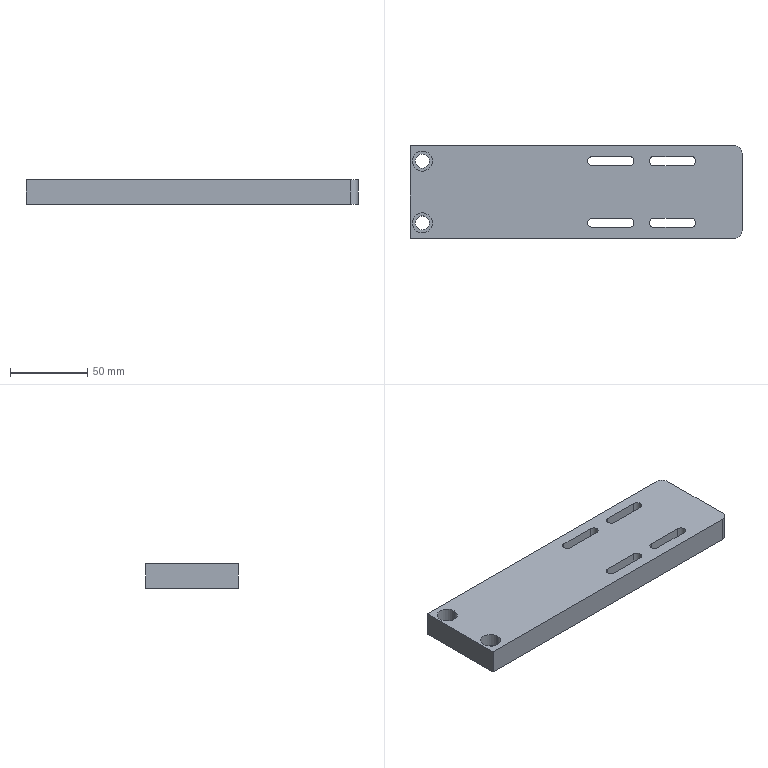NC program | Mastercam | posted with a generic post | part box 215 x 60 x 16 mm
Lines 5150 to 6620 of 6620, first 1383 of 1471 lines:
N1990 T7 M6
N2000 G0 G90 G17 G54 X-99.5 Y-20. A0. S3000 M3
N2010 G43 H7 Z50. M8
N2020 G98 G81 Z-.7 R1. F300.
N2030 Y20.
N2040 X10.5
N2050 X34.5
N2060 X50.5
N2070 X74.5
N2080 Y-20.
N2090 X50.5
N2100 X34.5
N2110 X10.5
N2120 G80
N2130 M5
N2140 G91 G0 G28 Z0. M9
N2150 A0.
N2160 M01
N2170 T1 M6
N2180 G0 G90 G17 G54 X-99.5 Y-20. A0. S2000 M3
N2190 G43 H1 Z50. M8
N2200 G98 G83 Z-18.902 R1. Q3. F200.
N2210 Y20.
N2220 X10.5
N2230 X34.5
N2240 X50.5
N2250 X74.5
N2260 Y-20.
N2270 X50.5
N2280 X34.5
N2290 X10.5
N2300 G80
N2310 M5
N2320 G91 G0 G28 Z0. M9
N2330 A0.
N2340 M01
N2350 T6 M6
N2360 G0 G90 G17 G54 X-99.5 Y20. A0. S7000 M3
N2370 G43 H6 Z50. M8
N2380 Z5.
N2390 G1 Z0. F600.
N2400 X-97.8 Y21.7 F3000.
N2410 G3 X-99.5 Y23.4 I-1.7 J0.
N2420 X-102.9 Y20. Z-.125 I0. J-3.4
N2430 X-99.5 Y16.6 Z-.25 I3.4 J0.
N2440 X-96.1 Y20. Z-.375 I0. J3.4
N2450 X-99.5 Y23.4 Z-.5 I-3.4 J0.
N2460 X-102.9 Y20. Z-.625 I0. J-3.4
N2470 X-99.5 Y16.6 Z-.75 I3.4 J0.
N2480 X-96.1 Y20. Z-.875 I0. J3.4
N2490 X-99.5 Y23.4 Z-1. I-3.4 J0.
N2500 X-102.9 Y20. Z-1.125 I0. J-3.4
N2510 X-99.5 Y16.6 Z-1.25 I3.4 J0.
N2520 X-96.1 Y20. Z-1.375 I0. J3.4
N2530 X-99.5 Y23.4 Z-1.5 I-3.4 J0.
N2540 X-102.9 Y20. Z-1.625 I0. J-3.4
N2550 X-99.5 Y16.6 Z-1.75 I3.4 J0.
N2560 X-96.1 Y20. Z-1.875 I0. J3.4
N2570 X-99.5 Y23.4 Z-2. I-3.4 J0.
N2580 X-102.9 Y20. Z-2.125 I0. J-3.4
N2590 X-99.5 Y16.6 Z-2.25 I3.4 J0.
N2600 X-96.1 Y20. Z-2.375 I0. J3.4
N2610 X-99.5 Y23.4 Z-2.5 I-3.4 J0.
N2620 X-102.9 Y20. Z-2.625 I0. J-3.4
N2630 X-99.5 Y16.6 Z-2.75 I3.4 J0.
N2640 X-96.1 Y20. Z-2.875 I0. J3.4
N2650 X-99.5 Y23.4 Z-3. I-3.4 J0.
N2660 X-102.9 Y20. Z-3.125 I0. J-3.4
N2670 X-99.5 Y16.6 Z-3.25 I3.4 J0.
N2680 X-96.1 Y20. Z-3.375 I0. J3.4
N2690 X-99.5 Y23.4 Z-3.5 I-3.4 J0.
N2700 X-102.9 Y20. Z-3.625 I0. J-3.4
N2710 X-99.5 Y16.6 Z-3.75 I3.4 J0.
N2720 X-96.1 Y20. Z-3.875 I0. J3.4
N2730 X-99.5 Y23.4 Z-4. I-3.4 J0.
N2740 X-102.9 Y20. Z-4.125 I0. J-3.4
N2750 X-99.5 Y16.6 Z-4.25 I3.4 J0.
N2760 X-96.1 Y20. Z-4.375 I0. J3.4
N2770 X-99.5 Y23.4 Z-4.5 I-3.4 J0.
N2780 X-102.9 Y20. Z-4.625 I0. J-3.4
N2790 X-99.5 Y16.6 Z-4.75 I3.4 J0.
N2800 X-96.1 Y20. Z-4.875 I0. J3.4
N2810 X-99.5 Y23.4 Z-5. I-3.4 J0.
N2820 X-102.9 Y20. Z-5.125 I0. J-3.4
N2830 X-99.5 Y16.6 Z-5.25 I3.4 J0.
N2840 X-96.1 Y20. Z-5.375 I0. J3.4
N2850 X-99.5 Y23.4 Z-5.5 I-3.4 J0.
N2860 X-102.9 Y20. Z-5.625 I0. J-3.4
N2870 X-99.5 Y16.6 Z-5.75 I3.4 J0.
N2880 X-96.1 Y20. Z-5.875 I0. J3.4
N2890 X-99.5 Y23.4 Z-6. I-3.4 J0.
N2900 X-102.9 Y20. Z-6.125 I0. J-3.4
N2910 X-99.5 Y16.6 Z-6.25 I3.4 J0.
N2920 X-96.1 Y20. Z-6.375 I0. J3.4
N2930 X-99.5 Y23.4 Z-6.5 I-3.4 J0.
N2940 X-102.9 Y20. Z-6.625 I0. J-3.4
N2950 X-99.5 Y16.6 Z-6.75 I3.4 J0.
N2960 X-96.1 Y20. Z-6.875 I0. J3.4
N2970 X-99.5 Y23.4 Z-7. I-3.4 J0.
N2980 X-102.9 Y20. Z-7.125 I0. J-3.4
N2990 X-99.5 Y16.6 Z-7.25 I3.4 J0.
N3000 X-96.1 Y20. Z-7.375 I0. J3.4
N3010 X-99.5 Y23.4 Z-7.5 I-3.4 J0.
N3020 X-102.9 Y20. Z-7.625 I0. J-3.4
N3030 X-99.5 Y16.6 Z-7.75 I3.4 J0.
N3040 X-96.1 Y20. Z-7.875 I0. J3.4
N3050 X-99.5 Y23.4 Z-8. I-3.4 J0.
N3060 X-102.9 Y20. Z-8.125 I0. J-3.4
N3070 X-99.5 Y16.6 Z-8.25 I3.4 J0.
N3080 X-96.1 Y20. Z-8.375 I0. J3.4
N3090 X-99.5 Y23.4 Z-8.5 I-3.4 J0.
N3100 X-102.9 Y20. Z-8.625 I0. J-3.4
N3110 X-99.5 Y16.6 Z-8.75 I3.4 J0.
N3120 X-96.1 Y20. Z-8.875 I0. J3.4
N3130 X-99.5 Y23.4 Z-9. I-3.4 J0.
N3140 X-102.9 Y20. I0. J-3.4 F900.
N3150 X-99.5 Y16.6 I3.4 J0.
N3160 X-96.1 Y20. I0. J3.4
N3170 X-99.5 Y23.4 I-3.4 J0.
N3180 X-100.486 Y23.254 I0. J-3.4
N3190 X-101.693 Y21.627 I.493 J-1.627
N3200 X-101.62 Y21.134 I1.7 J0.
N3210 G1 X-99.5 Y20.
N3220 G0 Z0.
N3230 G1 X-97.75 Y21.75 F1000.
N3240 G3 X-99.5 Y23.5 I-1.75 J0.
N3250 X-103. Y20. I0. J-3.5
N3260 X-99.5 Y16.5 I3.5 J0.
N3270 X-96. Y20. I0. J3.5
N3280 X-99.5 Y23.5 I-3.5 J0.
N3290 X-100.486 Y23.358 I0. J-3.5
N3300 X-103. Y20. Z-1.023 I.986 J-3.358
N3310 X-99.5 Y16.5 Z-2.273 I3.5 J0.
N3320 X-96. Y20. Z-3.523 I0. J3.5
N3330 X-99.5 Y23.5 Z-4.773 I-3.5 J0.
N3340 X-100.486 Y23.358 Z-5. I0. J-3.5
N3350 X-103. Y20. Z-6.023 I.986 J-3.358
N3360 X-99.5 Y16.5 Z-7.273 I3.5 J0.
N3370 X-96. Y20. Z-8.523 I0. J3.5
N3380 X-96.611 Y21.976 Z-9. I-3.5 J0.
N3390 X-99.5 Y23.5 I-2.889 J-1.976
N3400 X-103. Y20. I0. J-3.5
N3410 X-99.5 Y16.5 I3.5 J0.
N3420 X-96. Y20. I0. J3.5
N3430 X-96.611 Y21.976 I-3.5 J0.
N3440 X-97.285 Y22.71 I-2.889 J-1.976
N3450 X-98.393 Y23.105 I-1.108 J-1.355
N3460 X-99.748 Y22.462 I0. J-1.75
N3470 G1 X-99.5 Y20.
N3480 G0 Z50.
N3490 Y-20.
N3500 Z5.
N3510 G1 Z0. F600.
N3520 X-97.8 Y-18.3 F3000.
N3530 G3 X-99.5 Y-16.6 I-1.7 J0.
N3540 X-102.9 Y-20. Z-.125 I0. J-3.4
N3550 X-99.5 Y-23.4 Z-.25 I3.4 J0.
N3560 X-96.1 Y-20. Z-.375 I0. J3.4
N3570 X-99.5 Y-16.6 Z-.5 I-3.4 J0.
N3580 X-102.9 Y-20. Z-.625 I0. J-3.4
N3590 X-99.5 Y-23.4 Z-.75 I3.4 J0.
N3600 X-96.1 Y-20. Z-.875 I0. J3.4
N3610 X-99.5 Y-16.6 Z-1. I-3.4 J0.
N3620 X-102.9 Y-20. Z-1.125 I0. J-3.4
N3630 X-99.5 Y-23.4 Z-1.25 I3.4 J0.
N3640 X-96.1 Y-20. Z-1.375 I0. J3.4
N3650 X-99.5 Y-16.6 Z-1.5 I-3.4 J0.
N3660 X-102.9 Y-20. Z-1.625 I0. J-3.4
N3670 X-99.5 Y-23.4 Z-1.75 I3.4 J0.
N3680 X-96.1 Y-20. Z-1.875 I0. J3.4
N3690 X-99.5 Y-16.6 Z-2. I-3.4 J0.
N3700 X-102.9 Y-20. Z-2.125 I0. J-3.4
N3710 X-99.5 Y-23.4 Z-2.25 I3.4 J0.
N3720 X-96.1 Y-20. Z-2.375 I0. J3.4
N3730 X-99.5 Y-16.6 Z-2.5 I-3.4 J0.
N3740 X-102.9 Y-20. Z-2.625 I0. J-3.4
N3750 X-99.5 Y-23.4 Z-2.75 I3.4 J0.
N3760 X-96.1 Y-20. Z-2.875 I0. J3.4
N3770 X-99.5 Y-16.6 Z-3. I-3.4 J0.
N3780 X-102.9 Y-20. Z-3.125 I0. J-3.4
N3790 X-99.5 Y-23.4 Z-3.25 I3.4 J0.
N3800 X-96.1 Y-20. Z-3.375 I0. J3.4
N3810 X-99.5 Y-16.6 Z-3.5 I-3.4 J0.
N3820 X-102.9 Y-20. Z-3.625 I0. J-3.4
N3830 X-99.5 Y-23.4 Z-3.75 I3.4 J0.
N3840 X-96.1 Y-20. Z-3.875 I0. J3.4
N3850 X-99.5 Y-16.6 Z-4. I-3.4 J0.
N3860 X-102.9 Y-20. Z-4.125 I0. J-3.4
N3870 X-99.5 Y-23.4 Z-4.25 I3.4 J0.
N3880 X-96.1 Y-20. Z-4.375 I0. J3.4
N3890 X-99.5 Y-16.6 Z-4.5 I-3.4 J0.
N3900 X-102.9 Y-20. Z-4.625 I0. J-3.4
N3910 X-99.5 Y-23.4 Z-4.75 I3.4 J0.
N3920 X-96.1 Y-20. Z-4.875 I0. J3.4
N3930 X-99.5 Y-16.6 Z-5. I-3.4 J0.
N3940 X-102.9 Y-20. Z-5.125 I0. J-3.4
N3950 X-99.5 Y-23.4 Z-5.25 I3.4 J0.
N3960 X-96.1 Y-20. Z-5.375 I0. J3.4
N3970 X-99.5 Y-16.6 Z-5.5 I-3.4 J0.
N3980 X-102.9 Y-20. Z-5.625 I0. J-3.4
N3990 X-99.5 Y-23.4 Z-5.75 I3.4 J0.
N4000 X-96.1 Y-20. Z-5.875 I0. J3.4
N4010 X-99.5 Y-16.6 Z-6. I-3.4 J0.
N4020 X-102.9 Y-20. Z-6.125 I0. J-3.4
N4030 X-99.5 Y-23.4 Z-6.25 I3.4 J0.
N4040 X-96.1 Y-20. Z-6.375 I0. J3.4
N4050 X-99.5 Y-16.6 Z-6.5 I-3.4 J0.
N4060 X-102.9 Y-20. Z-6.625 I0. J-3.4
N4070 X-99.5 Y-23.4 Z-6.75 I3.4 J0.
N4080 X-96.1 Y-20. Z-6.875 I0. J3.4
N4090 X-99.5 Y-16.6 Z-7. I-3.4 J0.
N4100 X-102.9 Y-20. Z-7.125 I0. J-3.4
N4110 X-99.5 Y-23.4 Z-7.25 I3.4 J0.
N4120 X-96.1 Y-20. Z-7.375 I0. J3.4
N4130 X-99.5 Y-16.6 Z-7.5 I-3.4 J0.
N4140 X-102.9 Y-20. Z-7.625 I0. J-3.4
N4150 X-99.5 Y-23.4 Z-7.75 I3.4 J0.
N4160 X-96.1 Y-20. Z-7.875 I0. J3.4
N4170 X-99.5 Y-16.6 Z-8. I-3.4 J0.
N4180 X-102.9 Y-20. Z-8.125 I0. J-3.4
N4190 X-99.5 Y-23.4 Z-8.25 I3.4 J0.
N4200 X-96.1 Y-20. Z-8.375 I0. J3.4
N4210 X-99.5 Y-16.6 Z-8.5 I-3.4 J0.
N4220 X-102.9 Y-20. Z-8.625 I0. J-3.4
N4230 X-99.5 Y-23.4 Z-8.75 I3.4 J0.
N4240 X-96.1 Y-20. Z-8.875 I0. J3.4
N4250 X-99.5 Y-16.6 Z-9. I-3.4 J0.
N4260 X-102.9 Y-20. I0. J-3.4 F900.
N4270 X-99.5 Y-23.4 I3.4 J0.
N4280 X-96.1 Y-20. I0. J3.4
N4290 X-99.5 Y-16.6 I-3.4 J0.
N4300 X-100.486 Y-16.746 I0. J-3.4
N4310 X-101.693 Y-18.373 I.493 J-1.627
N4320 X-101.62 Y-18.866 I1.7 J0.
N4330 G1 X-99.5 Y-20.
N4340 G0 Z0.
N4350 G1 X-97.75 Y-18.25 F1000.
N4360 G3 X-99.5 Y-16.5 I-1.75 J0.
N4370 X-103. Y-20. I0. J-3.5
N4380 X-99.5 Y-23.5 I3.5 J0.
N4390 X-96. Y-20. I0. J3.5
N4400 X-99.5 Y-16.5 I-3.5 J0.
N4410 X-100.486 Y-16.642 I0. J-3.5
N4420 X-103. Y-20. Z-1.023 I.986 J-3.358
N4430 X-99.5 Y-23.5 Z-2.273 I3.5 J0.
N4440 X-96. Y-20. Z-3.523 I0. J3.5
N4450 X-99.5 Y-16.5 Z-4.773 I-3.5 J0.
N4460 X-100.486 Y-16.642 Z-5. I0. J-3.5
N4470 X-103. Y-20. Z-6.023 I.986 J-3.358
N4480 X-99.5 Y-23.5 Z-7.273 I3.5 J0.
N4490 X-96. Y-20. Z-8.523 I0. J3.5
N4500 X-96.611 Y-18.024 Z-9. I-3.5 J0.
N4510 X-99.5 Y-16.5 I-2.889 J-1.976
N4520 X-103. Y-20. I0. J-3.5
N4530 X-99.5 Y-23.5 I3.5 J0.
N4540 X-96. Y-20. I0. J3.5
N4550 X-96.611 Y-18.024 I-3.5 J0.
N4560 X-97.285 Y-17.29 I-2.889 J-1.976
N4570 X-98.393 Y-16.895 I-1.108 J-1.355
N4580 X-99.748 Y-17.538 I0. J-1.75
N4590 G1 X-99.5 Y-20.
N4600 G0 Z50.
N4610 M5
N4620 G91 G28 Z0. M9
N4630 A0.
N4640 M01
N4650 T5 M6
N4660 G0 G90 G17 G54 X10.5 Y20. A0. S7000 M3
N4670 G43 H5 Z25. M8
N4680 Z1.
N4690 G1 Z-.5 F600.
N4700 X34.5 F3000.
N4710 Z-1. F600.
N4720 X10.5 F3000.
N4730 Z-1.5 F600.
N4740 X34.5 F3000.
N4750 Z-2. F600.
N4760 X10.5 F3000.
N4770 Z-2.5 F600.
N4780 X34.5 F3000.
N4790 Z-3. F600.
N4800 X10.5 F3000.
N4810 Z-3.5 F600.
N4820 X34.5 F3000.
N4830 Z-4. F600.
N4840 X10.5 F3000.
N4850 Z-4.5 F600.
N4860 X34.5 F3000.
N4870 Z-5. F600.
N4880 X10.5 F3000.
N4890 Z-5.5 F600.
N4900 X34.5 F3000.
N4910 Z-6. F600.
N4920 X10.5 F3000.
N4930 Z-6.5 F600.
N4940 X34.5 F3000.
N4950 Z-7. F600.
N4960 X10.5 F3000.
N4970 Z-7.5 F600.
N4980 X34.5 F3000.
N4990 Z-8. F600.
N5000 X10.5 F3000.
N5010 Z-8.5 F600.
N5020 X34.5 F3000.
N5030 Z-9. F600.
N5040 X10.5 F3000.
N5050 Z-9.5 F600.
N5060 X34.5 F3000.
N5070 Z-10. F600.
N5080 X10.5 F3000.
N5090 Z-10.5 F600.
N5100 X34.5 F3000.
N5110 Z-11. F600.
N5120 X10.5 F3000.
N5130 Z-11.5 F600.
N5140 X34.5 F3000.
N5150 Z-12. F600.
N5160 X10.5 F3000.
N5170 Z-12.5 F600.
N5180 X34.5 F3000.
N5190 Z-13. F600.
N5200 X10.5 F3000.
N5210 Z-13.5 F600.
N5220 X34.5 F3000.
N5230 Z-14. F600.
N5240 X10.5 F3000.
N5250 Z-14.5 F600.
N5260 X34.5 F3000.
N5270 Z-15. F600.
N5280 X10.5 F3000.
N5290 Z-15.5 F600.
N5300 X34.5 F3000.
N5310 Z-16. F600.
N5320 X10.5 F3000.
N5330 Z-16.5 F600.
N5340 X34.5 F3000.
N5350 Z-17. F600.
N5360 X10.5 F3000.
N5370 G0 Z25.
N5380 X50.5
N5390 Z1.
N5400 G1 Z-.5 F600.
N5410 X74.5 F3000.
N5420 Z-1. F600.
N5430 X50.5 F3000.
N5440 Z-1.5 F600.
N5450 X74.5 F3000.
N5460 Z-2. F600.
N5470 X50.5 F3000.
N5480 Z-2.5 F600.
N5490 X74.5 F3000.
N5500 Z-3. F600.
N5510 X50.5 F3000.
N5520 Z-3.5 F600.
N5530 X74.5 F3000.
N5540 Z-4. F600.
N5550 X50.5 F3000.
N5560 Z-4.5 F600.
N5570 X74.5 F3000.
N5580 Z-5. F600.
N5590 X50.5 F3000.
N5600 Z-5.5 F600.
N5610 X74.5 F3000.
N5620 Z-6. F600.
N5630 X50.5 F3000.
N5640 Z-6.5 F600.
N5650 X74.5 F3000.
N5660 Z-7. F600.
N5670 X50.5 F3000.
N5680 Z-7.5 F600.
N5690 X74.5 F3000.
N5700 Z-8. F600.
N5710 X50.5 F3000.
N5720 Z-8.5 F600.
N5730 X74.5 F3000.
N5740 Z-9. F600.
N5750 X50.5 F3000.
N5760 Z-9.5 F600.
N5770 X74.5 F3000.
N5780 Z-10. F600.
N5790 X50.5 F3000.
N5800 Z-10.5 F600.
N5810 X74.5 F3000.
N5820 Z-11. F600.
N5830 X50.5 F3000.
N5840 Z-11.5 F600.
N5850 X74.5 F3000.
N5860 Z-12. F600.
N5870 X50.5 F3000.
N5880 Z-12.5 F600.
N5890 X74.5 F3000.
N5900 Z-13. F600.
N5910 X50.5 F3000.
N5920 Z-13.5 F600.
N5930 X74.5 F3000.
N5940 Z-14. F600.
N5950 X50.5 F3000.
N5960 Z-14.5 F600.
N5970 X74.5 F3000.
N5980 Z-15. F600.
N5990 X50.5 F3000.
N6000 Z-15.5 F600.
N6010 X74.5 F3000.
N6020 Z-16. F600.
N6030 X50.5 F3000.
N6040 Z-16.5 F600.
N6050 X74.5 F3000.
N6060 Z-17. F600.
N6070 X50.5 F3000.
N6080 G0 Z25.
N6090 X10.5 Y-20.
N6100 Z1.
N6110 G1 Z-.5 F600.
N6120 X34.5 F3000.
N6130 Z-1. F600.
N6140 X10.5 F3000.
N6150 Z-1.5 F600.
N6160 X34.5 F3000.
N6170 Z-2. F600.
N6180 X10.5 F3000.
N6190 Z-2.5 F600.
N6200 X34.5 F3000.
N6210 Z-3. F600.
N6220 X10.5 F3000.
N6230 Z-3.5 F600.
N6240 X34.5 F3000.
N6250 Z-4. F600.
N6260 X10.5 F3000.
N6270 Z-4.5 F600.
N6280 X34.5 F3000.
N6290 Z-5. F600.
N6300 X10.5 F3000.
N6310 Z-5.5 F600.
N6320 X34.5 F3000.
N6330 Z-6. F600.
N6340 X10.5 F3000.
N6350 Z-6.5 F600.
N6360 X34.5 F3000.
N6370 Z-7. F600.
N6380 X10.5 F3000.
N6390 Z-7.5 F600.
N6400 X34.5 F3000.
N6410 Z-8. F600.
N6420 X10.5 F3000.
N6430 Z-8.5 F600.
N6440 X34.5 F3000.
N6450 Z-9. F600.
N6460 X10.5 F3000.
N6470 Z-9.5 F600.
N6480 X34.5 F3000.
N6490 Z-10. F600.
N6500 X10.5 F3000.
N6510 Z-10.5 F600.
N6520 X34.5 F3000.
N6530 Z-11. F600.
N6540 X10.5 F3000.
N6550 Z-11.5 F600.
N6560 X34.5 F3000.
N6570 Z-12. F600.
N6580 X10.5 F3000.
N6590 Z-12.5 F600.
N6600 X34.5 F3000.
N6610 Z-13. F600.
N6620 X10.5 F3000.
N6630 Z-13.5 F600.
N6640 X34.5 F3000.
N6650 Z-14. F600.
N6660 X10.5 F3000.
N6670 Z-14.5 F600.
N6680 X34.5 F3000.
N6690 Z-15. F600.
N6700 X10.5 F3000.
N6710 Z-15.5 F600.
N6720 X34.5 F3000.
N6730 Z-16. F600.
N6740 X10.5 F3000.
N6750 Z-16.5 F600.
N6760 X34.5 F3000.
N6770 Z-17. F600.
N6780 X10.5 F3000.
N6790 G0 Z25.
N6800 X50.5
N6810 Z1.
N6820 G1 Z-.5 F600.
N6830 X74.5 F3000.
N6840 Z-1. F600.
N6850 X50.5 F3000.
N6860 Z-1.5 F600.
N6870 X74.5 F3000.
N6880 Z-2. F600.
N6890 X50.5 F3000.
N6900 Z-2.5 F600.
N6910 X74.5 F3000.
N6920 Z-3. F600.
N6930 X50.5 F3000.
N6940 Z-3.5 F600.
N6950 X74.5 F3000.
N6960 Z-4. F600.
N6970 X50.5 F3000.
N6980 Z-4.5 F600.
N6990 X74.5 F3000.
N7000 Z-5. F600.
N7010 X50.5 F3000.
N7020 Z-5.5 F600.
N7030 X74.5 F3000.
N7040 Z-6. F600.
N7050 X50.5 F3000.
N7060 Z-6.5 F600.
N7070 X74.5 F3000.
N7080 Z-7. F600.
N7090 X50.5 F3000.
N7100 Z-7.5 F600.
N7110 X74.5 F3000.
N7120 Z-8. F600.
N7130 X50.5 F3000.
N7140 Z-8.5 F600.
N7150 X74.5 F3000.
N7160 Z-9. F600.
N7170 X50.5 F3000.
N7180 Z-9.5 F600.
N7190 X74.5 F3000.
N7200 Z-10. F600.
N7210 X50.5 F3000.
N7220 Z-10.5 F600.
N7230 X74.5 F3000.
N7240 Z-11. F600.
N7250 X50.5 F3000.
N7260 Z-11.5 F600.
N7270 X74.5 F3000.
N7280 Z-12. F600.
N7290 X50.5 F3000.
N7300 Z-12.5 F600.
N7310 X74.5 F3000.
N7320 Z-13. F600.
N7330 X50.5 F3000.
N7340 Z-13.5 F600.
N7350 X74.5 F3000.
N7360 Z-14. F600.
N7370 X50.5 F3000.
N7380 Z-14.5 F600.
N7390 X74.5 F3000.
N7400 Z-15. F600.
N7410 X50.5 F3000.
N7420 Z-15.5 F600.
N7430 X74.5 F3000.
N7440 Z-16. F600.
N7450 X50.5 F3000.
N7460 Z-16.5 F600.
N7470 X74.5 F3000.
N7480 Z-17. F600.
N7490 X50.5 F3000.
N7500 G0 Z25.
N7510 X-99.5 Y20. Z41.
N7520 Z-4.
N7530 G1 Z-9. F600.
N7540 X-98.55 Y20.95 F3000.
N7550 G3 X-99.5 Y21.9 I-.95 J0.
N7560 X-101.4 Y20. Z-9.125 I0. J-1.9
N7570 X-99.5 Y18.1 Z-9.25 I1.9 J0.
N7580 X-97.6 Y20. Z-9.375 I0. J1.9
N7590 X-99.5 Y21.9 Z-9.5 I-1.9 J0.
N7600 X-101.4 Y20. Z-9.625 I0. J-1.9
N7610 X-99.5 Y18.1 Z-9.75 I1.9 J0.
N7620 X-97.6 Y20. Z-9.875 I0. J1.9
N7630 X-99.5 Y21.9 Z-10. I-1.9 J0.
N7640 X-101.4 Y20. Z-10.125 I0. J-1.9
N7650 X-99.5 Y18.1 Z-10.25 I1.9 J0.
N7660 X-97.6 Y20. Z-10.375 I0. J1.9
N7670 X-99.5 Y21.9 Z-10.5 I-1.9 J0.
N7680 X-101.4 Y20. Z-10.625 I0. J-1.9
N7690 X-99.5 Y18.1 Z-10.75 I1.9 J0.
N7700 X-97.6 Y20. Z-10.875 I0. J1.9
N7710 X-99.5 Y21.9 Z-11. I-1.9 J0.
N7720 X-101.4 Y20. Z-11.125 I0. J-1.9
N7730 X-99.5 Y18.1 Z-11.25 I1.9 J0.
N7740 X-97.6 Y20. Z-11.375 I0. J1.9
N7750 X-99.5 Y21.9 Z-11.5 I-1.9 J0.
N7760 X-101.4 Y20. Z-11.625 I0. J-1.9
N7770 X-99.5 Y18.1 Z-11.75 I1.9 J0.
N7780 X-97.6 Y20. Z-11.875 I0. J1.9
N7790 X-99.5 Y21.9 Z-12. I-1.9 J0.
N7800 X-101.4 Y20. Z-12.125 I0. J-1.9
N7810 X-99.5 Y18.1 Z-12.25 I1.9 J0.
N7820 X-97.6 Y20. Z-12.375 I0. J1.9
N7830 X-99.5 Y21.9 Z-12.5 I-1.9 J0.
N7840 X-101.4 Y20. Z-12.625 I0. J-1.9
N7850 X-99.5 Y18.1 Z-12.75 I1.9 J0.
N7860 X-97.6 Y20. Z-12.875 I0. J1.9
N7870 X-99.5 Y21.9 Z-13. I-1.9 J0.
N7880 X-101.4 Y20. Z-13.125 I0. J-1.9
N7890 X-99.5 Y18.1 Z-13.25 I1.9 J0.
N7900 X-97.6 Y20. Z-13.375 I0. J1.9
N7910 X-99.5 Y21.9 Z-13.5 I-1.9 J0.
N7920 X-101.4 Y20. Z-13.625 I0. J-1.9
N7930 X-99.5 Y18.1 Z-13.75 I1.9 J0.
N7940 X-97.6 Y20. Z-13.875 I0. J1.9
N7950 X-99.5 Y21.9 Z-14. I-1.9 J0.
N7960 X-101.4 Y20. Z-14.125 I0. J-1.9
N7970 X-99.5 Y18.1 Z-14.25 I1.9 J0.
N7980 X-97.6 Y20. Z-14.375 I0. J1.9
N7990 X-99.5 Y21.9 Z-14.5 I-1.9 J0.
N8000 X-101.4 Y20. Z-14.625 I0. J-1.9
N8010 X-99.5 Y18.1 Z-14.75 I1.9 J0.
N8020 X-97.6 Y20. Z-14.875 I0. J1.9
N8030 X-99.5 Y21.9 Z-15. I-1.9 J0.
N8040 X-101.4 Y20. Z-15.125 I0. J-1.9
N8050 X-99.5 Y18.1 Z-15.25 I1.9 J0.
N8060 X-97.6 Y20. Z-15.375 I0. J1.9
N8070 X-99.5 Y21.9 Z-15.5 I-1.9 J0.
N8080 X-101.4 Y20. Z-15.625 I0. J-1.9
N8090 X-99.5 Y18.1 Z-15.75 I1.9 J0.
N8100 X-97.6 Y20. Z-15.875 I0. J1.9
N8110 X-99.5 Y21.9 Z-16. I-1.9 J0.
N8120 X-101.4 Y20. Z-16.125 I0. J-1.9
N8130 X-99.5 Y18.1 Z-16.25 I1.9 J0.
N8140 X-97.6 Y20. Z-16.375 I0. J1.9
N8150 X-99.5 Y21.9 Z-16.5 I-1.9 J0.
N8160 X-101.4 Y20. Z-16.625 I0. J-1.9
N8170 X-99.5 Y18.1 Z-16.75 I1.9 J0.
N8180 X-97.6 Y20. Z-16.875 I0. J1.9
N8190 X-99.5 Y21.9 Z-17. I-1.9 J0.
N8200 X-101.4 Y20. I0. J-1.9 F900.
N8210 X-99.5 Y18.1 I1.9 J0.
N8220 X-97.6 Y20. I0. J1.9
N8230 X-99.5 Y21.9 I-1.9 J0.
N8240 X-100.454 Y21.643 I0. J-1.9
N8250 X-100.927 Y20.821 I.477 J-.822
N8260 X-100.799 Y20.344 I.95 J0.
N8270 G1 X-99.5 Y20.
N8280 G0 Z-9.
N8290 G1 X-98.5 Y21. F1000.
N8300 G3 X-99.5 Y22. I-1. J0.
N8310 X-101.5 Y20. I0. J-2.
N8320 X-99.5 Y18. I2. J0.
N8330 X-97.5 Y20. I0. J2.
N8340 X-99.5 Y22. I-2. J0.
N8350 X-100.459 Y21.755 I0. J-2.
N8360 X-101.5 Y20. Z-9.852 I.959 J-1.755
N8370 X-99.5 Y18. Z-11.102 I2. J0.
N8380 X-97.5 Y20. Z-12.352 I0. J2.
N8390 X-99.5 Y22. Z-13.602 I-2. J0.
N8400 X-100.459 Y21.755 Z-14. I0. J-2.
N8410 X-101.5 Y20. Z-14.852 I.959 J-1.755
N8420 X-99.5 Y18. Z-16.102 I2. J0.
N8430 X-97.693 Y19.144 Z-17. I0. J2.
N8440 X-97.501 Y20. I-1.807 J.856
N8450 X-99.5 Y21.999 I-1.999 J0.
N8460 X-101.499 Y20. I0. J-1.999
N8470 X-99.5 Y18.001 I1.999 J0.
N8480 X-97.693 Y19.144 I0. J1.999
N8490 X-97.501 Y20. I-1.807 J.856
N8500 X-97.503 Y20.115 I-1.999 J0.
N8510 X-98.502 Y21.058 I-.999 J-.058
N8520 X-98.559 Y21.056 I0. J-1.001
N8530 G1 X-99.5 Y20.
N8540 G0 Z41.
N8550 Y-20.
N8560 Z-4.
N8570 G1 Z-9. F600.
N8580 X-98.55 Y-19.05 F3000.
N8590 G3 X-99.5 Y-18.1 I-.95 J0.
N8600 X-101.4 Y-20. Z-9.125 I0. J-1.9
N8610 X-99.5 Y-21.9 Z-9.25 I1.9 J0.
N8620 X-97.6 Y-20. Z-9.375 I0. J1.9
N8630 X-99.5 Y-18.1 Z-9.5 I-1.9 J0.
N8640 X-101.4 Y-20. Z-9.625 I0. J-1.9
N8650 X-99.5 Y-21.9 Z-9.75 I1.9 J0.
N8660 X-97.6 Y-20. Z-9.875 I0. J1.9
N8670 X-99.5 Y-18.1 Z-10. I-1.9 J0.
N8680 X-101.4 Y-20. Z-10.125 I0. J-1.9
N8690 X-99.5 Y-21.9 Z-10.25 I1.9 J0.
N8700 X-97.6 Y-20. Z-10.375 I0. J1.9
N8710 X-99.5 Y-18.1 Z-10.5 I-1.9 J0.
N8720 X-101.4 Y-20. Z-10.625 I0. J-1.9
N8730 X-99.5 Y-21.9 Z-10.75 I1.9 J0.
N8740 X-97.6 Y-20. Z-10.875 I0. J1.9
N8750 X-99.5 Y-18.1 Z-11. I-1.9 J0.
N8760 X-101.4 Y-20. Z-11.125 I0. J-1.9
N8770 X-99.5 Y-21.9 Z-11.25 I1.9 J0.
N8780 X-97.6 Y-20. Z-11.375 I0. J1.9
N8790 X-99.5 Y-18.1 Z-11.5 I-1.9 J0.
N8800 X-101.4 Y-20. Z-11.625 I0. J-1.9
N8810 X-99.5 Y-21.9 Z-11.75 I1.9 J0.
N8820 X-97.6 Y-20. Z-11.875 I0. J1.9
N8830 X-99.5 Y-18.1 Z-12. I-1.9 J0.
N8840 X-101.4 Y-20. Z-12.125 I0. J-1.9
N8850 X-99.5 Y-21.9 Z-12.25 I1.9 J0.
N8860 X-97.6 Y-20. Z-12.375 I0. J1.9
N8870 X-99.5 Y-18.1 Z-12.5 I-1.9 J0.
N8880 X-101.4 Y-20. Z-12.625 I0. J-1.9
N8890 X-99.5 Y-21.9 Z-12.75 I1.9 J0.
N8900 X-97.6 Y-20. Z-12.875 I0. J1.9
N8910 X-99.5 Y-18.1 Z-13. I-1.9 J0.
N8920 X-101.4 Y-20. Z-13.125 I0. J-1.9
N8930 X-99.5 Y-21.9 Z-13.25 I1.9 J0.
N8940 X-97.6 Y-20. Z-13.375 I0. J1.9
N8950 X-99.5 Y-18.1 Z-13.5 I-1.9 J0.
N8960 X-101.4 Y-20. Z-13.625 I0. J-1.9
N8970 X-99.5 Y-21.9 Z-13.75 I1.9 J0.
N8980 X-97.6 Y-20. Z-13.875 I0. J1.9
N8990 X-99.5 Y-18.1 Z-14. I-1.9 J0.
N9000 X-101.4 Y-20. Z-14.125 I0. J-1.9
N9010 X-99.5 Y-21.9 Z-14.25 I1.9 J0.
N9020 X-97.6 Y-20. Z-14.375 I0. J1.9
N9030 X-99.5 Y-18.1 Z-14.5 I-1.9 J0.
N9040 X-101.4 Y-20. Z-14.625 I0. J-1.9
N9050 X-99.5 Y-21.9 Z-14.75 I1.9 J0.
N9060 X-97.6 Y-20. Z-14.875 I0. J1.9
N9070 X-99.5 Y-18.1 Z-15. I-1.9 J0.
N9080 X-101.4 Y-20. Z-15.125 I0. J-1.9
N9090 X-99.5 Y-21.9 Z-15.25 I1.9 J0.
N9100 X-97.6 Y-20. Z-15.375 I0. J1.9
N9110 X-99.5 Y-18.1 Z-15.5 I-1.9 J0.
N9120 X-101.4 Y-20. Z-15.625 I0. J-1.9
N9130 X-99.5 Y-21.9 Z-15.75 I1.9 J0.
N9140 X-97.6 Y-20. Z-15.875 I0. J1.9
N9150 X-99.5 Y-18.1 Z-16. I-1.9 J0.
N9160 X-101.4 Y-20. Z-16.125 I0. J-1.9
N9170 X-99.5 Y-21.9 Z-16.25 I1.9 J0.
N9180 X-97.6 Y-20. Z-16.375 I0. J1.9
N9190 X-99.5 Y-18.1 Z-16.5 I-1.9 J0.
N9200 X-101.4 Y-20. Z-16.625 I0. J-1.9
N9210 X-99.5 Y-21.9 Z-16.75 I1.9 J0.
N9220 X-97.6 Y-20. Z-16.875 I0. J1.9
N9230 X-99.5 Y-18.1 Z-17. I-1.9 J0.
N9240 X-101.4 Y-20. I0. J-1.9 F900.
N9250 X-99.5 Y-21.9 I1.9 J0.
N9260 X-97.6 Y-20. I0. J1.9
N9270 X-99.5 Y-18.1 I-1.9 J0.
N9280 X-100.454 Y-18.357 I0. J-1.9
N9290 X-100.927 Y-19.179 I.477 J-.822
N9300 X-100.799 Y-19.656 I.95 J0.
N9310 G1 X-99.5 Y-20.
N9320 G0 Z-9.
N9330 G1 X-98.5 Y-19. F1000.
N9340 G3 X-99.5 Y-18. I-1. J0.
N9350 X-101.5 Y-20. I0. J-2.
N9360 X-99.5 Y-22. I2. J0.
N9370 X-97.5 Y-20. I0. J2.
N9380 X-99.5 Y-18. I-2. J0.
N9390 X-100.459 Y-18.245 I0. J-2.
N9400 X-101.5 Y-20. Z-9.852 I.959 J-1.755
N9410 X-99.5 Y-22. Z-11.102 I2. J0.
N9420 X-97.5 Y-20. Z-12.352 I0. J2.
N9430 X-99.5 Y-18. Z-13.602 I-2. J0.
N9440 X-100.459 Y-18.245 Z-14. I0. J-2.
N9450 X-101.5 Y-20. Z-14.852 I.959 J-1.755
N9460 X-99.5 Y-22. Z-16.102 I2. J0.
N9470 X-97.693 Y-20.856 Z-17. I0. J2.
N9480 X-97.501 Y-20. I-1.807 J.856
N9490 X-99.5 Y-18.001 I-1.999 J0.
N9500 X-101.499 Y-20. I0. J-1.999
N9510 X-99.5 Y-21.999 I1.999 J0.
N9520 X-97.693 Y-20.856 I0. J1.999
N9530 X-97.501 Y-20. I-1.807 J.856
N9540 X-97.503 Y-19.885 I-1.999 J0.
N9550 X-98.502 Y-18.942 I-.999 J-.058
N9560 X-98.559 Y-18.944 I0. J-1.001
N9570 G1 X-99.5 Y-20.
N9580 G0 Z41.
N9590 X34.75 Y19.9 Z25.
N9600 Z1.
N9610 G1 Z0. F600.
N9620 Y20.15 F1500.
N9630 G3 X34.5 Y20.4 I-.25 J0.
N9640 G1 X10.5 Z-1.425
N9650 G3 X10.1 Y20. Z-1.463 I0. J-.4
N9660 X10.5 Y19.6 Z-1.5 I.4 J0.
N9670 G1 X34.5 Z-2.925
N9680 G3 X34.9 Y20. Z-2.962 I0. J.4
N9690 X34.5 Y20.4 Z-3. I-.4 J0.
N9700 G1 X10.5 Z-4.425
N9710 G3 X10.1 Y20. Z-4.463 I0. J-.4
N9720 X10.5 Y19.6 Z-4.5 I.4 J0.
N9730 G1 X34.5 Z-5.925
N9740 G3 X34.9 Y20. Z-5.963 I0. J.4
N9750 X34.5 Y20.4 Z-6. I-.4 J0.
N9760 G1 X10.5 Z-7.425
N9770 G3 X10.1 Y20. Z-7.463 I0. J-.4
N9780 X10.5 Y19.6 Z-7.5 I.4 J0.
N9790 G1 X34.5 Z-8.925
N9800 G3 X34.9 Y20. Z-8.963 I0. J.4
N9810 X34.5 Y20.4 Z-9. I-.4 J0.
N9820 G1 X10.5 Z-10.425
N9830 G3 X10.1 Y20. Z-10.463 I0. J-.4
N9840 X10.5 Y19.6 Z-10.5 I.4 J0.
N9850 G1 X34.5 Z-11.925
N9860 G3 X34.9 Y20. Z-11.963 I0. J.4
N9870 X34.5 Y20.4 Z-12. I-.4 J0.
N9880 G1 X10.5 Z-13.425
N9890 G3 X10.1 Y20. Z-13.463 I0. J-.4
N9900 X10.5 Y19.6 Z-13.5 I.4 J0.
N9910 G1 X34.5 Z-14.925
N9920 G3 X34.9 Y20. Z-14.963 I0. J.4
N9930 X34.5 Y20.4 Z-15. I-.4 J0.
N9940 G1 X10.5 Z-16.425
N9950 G3 X10.1 Y20. Z-16.463 I0. J-.4
N9960 X10.5 Y19.6 Z-16.5 I.4 J0.
N9970 G1 X18.919 Z-17.
N9980 X34.5
N9990 G3 X34.9 Y20. I0. J.4
N100 X34.5 Y20.4 I-.4 J0.
N110 G1 X10.5
N120 G3 X10.1 Y20. I0. J-.4
N130 X10.5 Y19.6 I.4 J0.
N140 G1 X19.419
N150 G3 X19.669 Y19.85 I0. J.25
N160 G1 Y20.1
N170 G0 Z25.
N180 X34.75 Y20.
N190 Z1.
N200 G1 Z0. F600.
N210 Y20.25 F1000.
N220 G3 X34.5 Y20.5 I-.25 J0.
N230 G1 X10.5 Z-1.408
N240 G3 X10. Y20. Z-1.454 I0. J-.5
N250 X10.5 Y19.5 Z-1.5 I.5 J0.
N260 G1 X34.5 Z-2.908
N270 G3 X35. Y20. Z-2.954 I0. J.5
N280 X34.5 Y20.5 Z-3. I-.5 J0.
N290 G1 X10.5 Z-4.408
N300 G3 X10. Y20. Z-4.454 I0. J-.5
N310 X10.5 Y19.5 Z-4.5 I.5 J0.
N320 G1 X34.5 Z-5.908
N330 G3 X35. Y20. Z-5.954 I0. J.5
N340 X34.5 Y20.5 Z-6. I-.5 J0.
N350 G1 X10.5 Z-7.408
N360 G3 X10. Y20. Z-7.454 I0. J-.5
N370 X10.5 Y19.5 Z-7.5 I.5 J0.
N380 G1 X34.5 Z-8.908
N390 G3 X35. Y20. Z-8.954 I0. J.5
N400 X34.5 Y20.5 Z-9. I-.5 J0.
N410 G1 X10.5 Z-10.408
N420 G3 X10. Y20. Z-10.454 I0. J-.5
N430 X10.5 Y19.5 Z-10.5 I.5 J0.
N440 G1 X34.5 Z-11.908
N450 G3 X35. Y20. Z-11.954 I0. J.5
N460 X34.5 Y20.5 Z-12. I-.5 J0.
N470 G1 X10.5 Z-13.408
N480 G3 X10. Y20. Z-13.454 I0. J-.5
N490 X10.5 Y19.5 Z-13.5 I.5 J0.
N500 G1 X34.5 Z-14.908
N510 G3 X35. Y20. Z-14.954 I0. J.5
N520 X34.5 Y20.5 Z-15. I-.5 J0.
N530 G1 X10.5 Z-16.408
N540 G3 X10. Y20. Z-16.454 I0. J-.5
N550 X10.5 Y19.5 Z-16.5 I.5 J0.
N560 G1 X19.024 Z-17.
N570 X34.5
N580 G3 X35. Y20. I0. J.5
N590 X34.5 Y20.5 I-.5 J0.
N600 G1 X10.5
N610 G3 X10. Y20. I0. J-.5
N620 X10.5 Y19.5 I.5 J0.
N630 G1 X19.524
N640 G3 X19.774 Y19.75 I0. J.25
N650 G1 Y20.
N660 G0 Z25.
N670 X74.75 Y19.9
N680 Z1.
N690 G1 Z0. F600.
N700 Y20.15 F1500.
N710 G3 X74.5 Y20.4 I-.25 J0.
N720 G1 X50.5 Z-1.425
N730 G3 X50.1 Y20. Z-1.463 I0. J-.4
N740 X50.5 Y19.6 Z-1.5 I.4 J0.
N750 G1 X74.5 Z-2.925
N760 G3 X74.9 Y20. Z-2.962 I0. J.4
N770 X74.5 Y20.4 Z-3. I-.4 J0.
N780 G1 X50.5 Z-4.425
N790 G3 X50.1 Y20. Z-4.463 I0. J-.4
N800 X50.5 Y19.6 Z-4.5 I.4 J0.
N810 G1 X74.5 Z-5.925
N820 G3 X74.9 Y20. Z-5.963 I0. J.4
N830 X74.5 Y20.4 Z-6. I-.4 J0.
N840 G1 X50.5 Z-7.425
N850 G3 X50.1 Y20. Z-7.463 I0. J-.4
N860 X50.5 Y19.6 Z-7.5 I.4 J0.
N870 G1 X74.5 Z-8.925
N880 G3 X74.9 Y20. Z-8.963 I0. J.4
N890 X74.5 Y20.4 Z-9. I-.4 J0.
N900 G1 X50.5 Z-10.425
N910 G3 X50.1 Y20. Z-10.463 I0. J-.4
N920 X50.5 Y19.6 Z-10.5 I.4 J0.
N930 G1 X74.5 Z-11.925
N940 G3 X74.9 Y20. Z-11.963 I0. J.4
N950 X74.5 Y20.4 Z-12. I-.4 J0.
N960 G1 X50.5 Z-13.425
N970 G3 X50.1 Y20. Z-13.463 I0. J-.4
N980 X50.5 Y19.6 Z-13.5 I.4 J0.
N990 G1 X74.5 Z-14.925
N1000 G3 X74.9 Y20. Z-14.963 I0. J.4
N1010 X74.5 Y20.4 Z-15. I-.4 J0.
N1020 G1 X50.5 Z-16.425
N1030 G3 X50.1 Y20. Z-16.463 I0. J-.4
N1040 X50.5 Y19.6 Z-16.5 I.4 J0.
N1050 G1 X58.919 Z-17.
N1060 X74.5
N1070 G3 X74.9 Y20. I0. J.4
N1080 X74.5 Y20.4 I-.4 J0.
N1090 G1 X50.5
N1100 G3 X50.1 Y20. I0. J-.4
N1110 X50.5 Y19.6 I.4 J0.
N1120 G1 X59.419
N1130 G3 X59.669 Y19.85 I0. J.25
N1140 G1 Y20.1
N1150 G0 Z25.
N1160 X74.75 Y20.
N1170 Z1.
N1180 G1 Z0. F600.
N1190 Y20.25 F1000.
N1200 G3 X74.5 Y20.5 I-.25 J0.
N1210 G1 X50.5 Z-1.408
N1220 G3 X50. Y20. Z-1.454 I0. J-.5
N1230 X50.5 Y19.5 Z-1.5 I.5 J0.
N1240 G1 X74.5 Z-2.908
N1250 G3 X75. Y20. Z-2.954 I0. J.5
N1260 X74.5 Y20.5 Z-3. I-.5 J0.
N1270 G1 X50.5 Z-4.408
N1280 G3 X50. Y20. Z-4.454 I0. J-.5
N1290 X50.5 Y19.5 Z-4.5 I.5 J0.
N1300 G1 X74.5 Z-5.908
N1310 G3 X75. Y20. Z-5.954 I0. J.5
N1320 X74.5 Y20.5 Z-6. I-.5 J0.
N1330 G1 X50.5 Z-7.408
N1340 G3 X50. Y20. Z-7.454 I0. J-.5
N1350 X50.5 Y19.5 Z-7.5 I.5 J0.
N1360 G1 X74.5 Z-8.908
N1370 G3 X75. Y20. Z-8.954 I0. J.5
N1380 X74.5 Y20.5 Z-9. I-.5 J0.
N1390 G1 X50.5 Z-10.408
N1400 G3 X50. Y20. Z-10.454 I0. J-.5
N1410 X50.5 Y19.5 Z-10.5 I.5 J0.
N1420 G1 X74.5 Z-11.908
N1430 G3 X75. Y20. Z-11.954 I0. J.5
N1440 X74.5 Y20.5 Z-12. I-.5 J0.
N1450 G1 X50.5 Z-13.408
N1460 G3 X50. Y20. Z-13.454 I0. J-.5
N1470 X50.5 Y19.5 Z-13.5 I.5 J0.
N1480 G1 X74.5 Z-14.908
N1490 G3 X75. Y20. Z-14.954 I0. J.5
N1500 X74.5 Y20.5 Z-15. I-.5 J0.
N1510 G1 X50.5 Z-16.408
N1520 G3 X50. Y20. Z-16.454 I0. J-.5
N1530 X50.5 Y19.5 Z-16.5 I.5 J0.
N1540 G1 X59.024 Z-17.
N1550 X74.5
N1560 G3 X75. Y20. I0. J.5
N1570 X74.5 Y20.5 I-.5 J0.
N1580 G1 X50.5
N1590 G3 X50. Y20. I0. J-.5
N1600 X50.5 Y19.5 I.5 J0.
N1610 G1 X59.524
N1620 G3 X59.774 Y19.75 I0. J.25
N1630 G1 Y20.
N1640 G0 Z25.
N1650 X74.75 Y-20.1
N1660 Z1.
N1670 G1 Z0. F600.
N1680 Y-19.85 F1500.
N1690 G3 X74.5 Y-19.6 I-.25 J0.
N1700 G1 X50.5 Z-1.425
N1710 G3 X50.1 Y-20. Z-1.463 I0. J-.4
N1720 X50.5 Y-20.4 Z-1.5 I.4 J0.
N1730 G1 X74.5 Z-2.925
N1740 G3 X74.9 Y-20. Z-2.962 I0. J.4
N1750 X74.5 Y-19.6 Z-3. I-.4 J0.
N1760 G1 X50.5 Z-4.425
N1770 G3 X50.1 Y-20. Z-4.463 I0. J-.4
N1780 X50.5 Y-20.4 Z-4.5 I.4 J0.
N1790 G1 X74.5 Z-5.925
N1800 G3 X74.9 Y-20. Z-5.963 I0. J.4
N1810 X74.5 Y-19.6 Z-6. I-.4 J0.
N1820 G1 X50.5 Z-7.425
N1830 G3 X50.1 Y-20. Z-7.463 I0. J-.4
N1840 X50.5 Y-20.4 Z-7.5 I.4 J0.
N1850 G1 X74.5 Z-8.925
N1860 G3 X74.9 Y-20. Z-8.963 I0. J.4
N1870 X74.5 Y-19.6 Z-9. I-.4 J0.
N1880 G1 X50.5 Z-10.425
N1890 G3 X50.1 Y-20. Z-10.463 I0. J-.4
N1900 X50.5 Y-20.4 Z-10.5 I.4 J0.
N1910 G1 X74.5 Z-11.925
N1920 G3 X74.9 Y-20. Z-11.963 I0. J.4
N1930 X74.5 Y-19.6 Z-12. I-.4 J0.
N1940 G1 X50.5 Z-13.425
N1950 G3 X50.1 Y-20. Z-13.463 I0. J-.4
N1960 X50.5 Y-20.4 Z-13.5 I.4 J0.
N1970 G1 X74.5 Z-14.925
N1980 G3 X74.9 Y-20. Z-14.963 I0. J.4
N1990 X74.5 Y-19.6 Z-15. I-.4 J0.
N2000 G1 X50.5 Z-16.425
N2010 G3 X50.1 Y-20. Z-16.463 I0. J-.4
N2020 X50.5 Y-20.4 Z-16.5 I.4 J0.
N2030 G1 X58.919 Z-17.
N2040 X74.5
N2050 G3 X74.9 Y-20. I0. J.4
N2060 X74.5 Y-19.6 I-.4 J0.
N2070 G1 X50.5
N2080 G3 X50.1 Y-20. I0. J-.4
N2090 X50.5 Y-20.4 I.4 J0.
N2100 G1 X59.419
N2110 G3 X59.669 Y-20.15 I0. J.25
N2120 G1 Y-19.9
N2130 G0 Z25.
N2140 X74.75 Y-20.
N2150 Z1.
N2160 G1 Z0. F600.
N2170 Y-19.75 F1000.
N2180 G3 X74.5 Y-19.5 I-.25 J0.
N2190 G1 X50.5 Z-1.408
N2200 G3 X50. Y-20. Z-1.454 I0. J-.5
N2210 X50.5 Y-20.5 Z-1.5 I.5 J0.
N2220 G1 X74.5 Z-2.908
N2230 G3 X75. Y-20. Z-2.954 I0. J.5
N2240 X74.5 Y-19.5 Z-3. I-.5 J0.
N2250 G1 X50.5 Z-4.408
N2260 G3 X50. Y-20. Z-4.454 I0. J-.5
N2270 X50.5 Y-20.5 Z-4.5 I.5 J0.
N2280 G1 X74.5 Z-5.908
N2290 G3 X75. Y-20. Z-5.954 I0. J.5
N2300 X74.5 Y-19.5 Z-6. I-.5 J0.
N2310 G1 X50.5 Z-7.408
N2320 G3 X50. Y-20. Z-7.454 I0. J-.5
N2330 X50.5 Y-20.5 Z-7.5 I.5 J0.
N2340 G1 X74.5 Z-8.908
N2350 G3 X75. Y-20. Z-8.954 I0. J.5
N2360 X74.5 Y-19.5 Z-9. I-.5 J0.
N2370 G1 X50.5 Z-10.408
N2380 G3 X50. Y-20. Z-10.454 I0. J-.5
N2390 X50.5 Y-20.5 Z-10.5 I.5 J0.
N2400 G1 X74.5 Z-11.908
N2410 G3 X75. Y-20. Z-11.954 I0. J.5
N2420 X74.5 Y-19.5 Z-12. I-.5 J0.
N2430 G1 X50.5 Z-13.408
N2440 G3 X50. Y-20. Z-13.454 I0. J-.5
N2450 X50.5 Y-20.5 Z-13.5 I.5 J0.
N2460 G1 X74.5 Z-14.908
N2470 G3 X75. Y-20. Z-14.954 I0. J.5
N2480 X74.5 Y-19.5 Z-15. I-.5 J0.
N2490 G1 X50.5 Z-16.408
N2500 G3 X50. Y-20. Z-16.454 I0. J-.5
N2510 X50.5 Y-20.5 Z-16.5 I.5 J0.
N2520 G1 X59.024 Z-17.
N2530 X74.5
N2540 G3 X75. Y-20. I0. J.5
N2550 X74.5 Y-19.5 I-.5 J0.
N2560 G1 X50.5
N2570 G3 X50. Y-20. I0. J-.5
N2580 X50.5 Y-20.5 I.5 J0.
N2590 G1 X59.524
N2600 G3 X59.774 Y-20.25 I0. J.25
N2610 G1 Y-20.
N2620 G0 Z25.
N2630 X34.75 Y-20.1
N2640 Z1.
N2650 G1 Z0. F600.
N2660 Y-19.85 F1500.
N2670 G3 X34.5 Y-19.6 I-.25 J0.
N2680 G1 X10.5 Z-1.425
N2690 G3 X10.1 Y-20. Z-1.463 I0. J-.4
N2700 X10.5 Y-20.4 Z-1.5 I.4 J0.
N2710 G1 X34.5 Z-2.925
N2720 G3 X34.9 Y-20. Z-2.962 I0. J.4
N2730 X34.5 Y-19.6 Z-3. I-.4 J0.
N2740 G1 X10.5 Z-4.425
N2750 G3 X10.1 Y-20. Z-4.463 I0. J-.4
N2760 X10.5 Y-20.4 Z-4.5 I.4 J0.
N2770 G1 X34.5 Z-5.925
N2780 G3 X34.9 Y-20. Z-5.963 I0. J.4
N2790 X34.5 Y-19.6 Z-6. I-.4 J0.
N2800 G1 X10.5 Z-7.425
N2810 G3 X10.1 Y-20. Z-7.463 I0. J-.4
N2820 X10.5 Y-20.4 Z-7.5 I.4 J0.
N2830 G1 X34.5 Z-8.925
N2840 G3 X34.9 Y-20. Z-8.963 I0. J.4
N2850 X34.5 Y-19.6 Z-9. I-.4 J0.
N2860 G1 X10.5 Z-10.425
N2870 G3 X10.1 Y-20. Z-10.463 I0. J-.4
N2880 X10.5 Y-20.4 Z-10.5 I.4 J0.
N2890 G1 X34.5 Z-11.925
N2900 G3 X34.9 Y-20. Z-11.963 I0. J.4
N2910 X34.5 Y-19.6 Z-12. I-.4 J0.
N2920 G1 X10.5 Z-13.425
N2930 G3 X10.1 Y-20. Z-13.463 I0. J-.4
N2940 X10.5 Y-20.4 Z-13.5 I.4 J0.
N2950 G1 X34.5 Z-14.925
N2960 G3 X34.9 Y-20. Z-14.963 I0. J.4
N2970 X34.5 Y-19.6 Z-15. I-.4 J0.
N2980 G1 X10.5 Z-16.425
N2990 G3 X10.1 Y-20. Z-16.463 I0. J-.4
N3000 X10.5 Y-20.4 Z-16.5 I.4 J0.
N3010 G1 X18.919 Z-17.
N3020 X34.5
N3030 G3 X34.9 Y-20. I0. J.4
N3040 X34.5 Y-19.6 I-.4 J0.
N3050 G1 X10.5
N3060 G3 X10.1 Y-20. I0. J-.4
N3070 X10.5 Y-20.4 I.4 J0.
N3080 G1 X19.419
N3090 G3 X19.669 Y-20.15 I0. J.25
N3100 G1 Y-19.9
N3110 G0 Z25.
N3120 X34.75 Y-20.
N3130 Z1.
N3140 G1 Z0. F600.
N3150 Y-19.75 F1000.
N3160 G3 X34.5 Y-19.5 I-.25 J0.
N3170 G1 X10.5 Z-1.408
N3180 G3 X10. Y-20. Z-1.454 I0. J-.5
N3190 X10.5 Y-20.5 Z-1.5 I.5 J0.
N3200 G1 X34.5 Z-2.908
N3210 G3 X35. Y-20. Z-2.954 I0. J.5
N3220 X34.5 Y-19.5 Z-3. I-.5 J0.
N3230 G1 X10.5 Z-4.408
N3240 G3 X10. Y-20. Z-4.454 I0. J-.5
N3250 X10.5 Y-20.5 Z-4.5 I.5 J0.
N3260 G1 X34.5 Z-5.908
N3270 G3 X35. Y-20. Z-5.954 I0. J.5
N3280 X34.5 Y-19.5 Z-6. I-.5 J0.
N3290 G1 X10.5 Z-7.408
N3300 G3 X10. Y-20. Z-7.454 I0. J-.5
N3310 X10.5 Y-20.5 Z-7.5 I.5 J0.
N3320 G1 X34.5 Z-8.908
N3330 G3 X35. Y-20. Z-8.954 I0. J.5
N3340 X34.5 Y-19.5 Z-9. I-.5 J0.
N3350 G1 X10.5 Z-10.408
N3360 G3 X10. Y-20. Z-10.454 I0. J-.5
N3370 X10.5 Y-20.5 Z-10.5 I.5 J0.
N3380 G1 X34.5 Z-11.908
N3390 G3 X35. Y-20. Z-11.954 I0. J.5
N3400 X34.5 Y-19.5 Z-12. I-.5 J0.
N3410 G1 X10.5 Z-13.408
N3420 G3 X10. Y-20. Z-13.454 I0. J-.5
N3430 X10.5 Y-20.5 Z-13.5 I.5 J0.
N3440 G1 X34.5 Z-14.908
N3450 G3 X35. Y-20. Z-14.954 I0. J.5
N3460 X34.5 Y-19.5 Z-15. I-.5 J0.
N3470 G1 X10.5 Z-16.408
N3480 G3 X10. Y-20. Z-16.454 I0. J-.5
N3490 X10.5 Y-20.5 Z-16.5 I.5 J0.
N3500 G1 X19.024 Z-17.
N3510 X34.5
N3520 G3 X35. Y-20. I0. J.5
N3530 X34.5 Y-19.5 I-.5 J0.
N3540 G1 X10.5
N3550 G3 X10. Y-20. I0. J-.5
N3560 X10.5 Y-20.5 I.5 J0.
N3570 G1 X19.524
N3580 G3 X19.774 Y-20.25 I0. J.25
N3590 G1 Y-20.
N3600 G0 Z25.
N3610 M5
N3620 G91 G28 Z0. M9
N3630 A0.
N3640 M01
N3650 T21 M6
N3660 G0 G90 G17 G54 X112.795 Y31.574 A0. S7000 M3
N3670 G43 H21 Z25. M8
N3680 Z-16.
N3690 G1 Z-17. F600.
N3700 X112.274 Y31.276 F1000.
N3710 G3 X111.972 Y30.755 I.298 J-.521
N3720 X112.051 Y30.457 I.6 J0.
N3730 G2 X113.5 Y25. I-9.551 J-5.457
N3740 G1 Y-25.
N3750 G2 X102.5 Y-36. I-11. J0.
N3760 G1 X-107.5
N3770 G2 X-113.5 Y-30. I0. J6.
N3780 G1 Y30.
N3790 G2 X-107.5 Y36. I6. J0.
N3800 G1 X102.5
N3810 G2 X112.289 Y30.018 I0. J-11.
N3820 G3 X112.823 Y29.691 I.534 J.273
N3830 X113.097 Y29.757 I0. J.6
N3840 G1 X113.63 Y30.031
N3850 G0 Z25.
N3860 M5
N3870 G91 G28 Z0. M9
N3880 A0.
N3890 M01
N3900 T7 M6
N3910 G0 G90 G17 G54 X35. Y-19.15 A0. S7000 M3
N3920 G43 H7 Z24.906 M8
N3930 Z24.7
N3940 Z-.3
N3950 G1 Z-1.3 F600.
N3960 Y-18.65 F1000.
N3970 G3 X34.5 Y-18.15 I-.5 J0.
N3980 G1 X10.5
N3990 G3 X8.65 Y-20. I0. J-1.85
N4000 X10.5 Y-21.85 I1.85 J0.
N4010 G1 X34.5
N4020 G3 X36.35 Y-20. I0. J1.85
N4030 X34.5 Y-18.15 I-1.85 J0.
N4040 X34. Y-18.65 I0. J-.5
N4050 G1 Y-19.15
N4060 G0 Z23.7
N4070 Z25.
N4080 X44.25
N4090 X75.
N4100 Z24.7
N4110 Z-.3
N4120 G1 Z-1.3 F600.
N4130 Y-18.65 F1000.
N4140 G3 X74.5 Y-18.15 I-.5 J0.
N4150 G1 X50.5
N4160 G3 X48.65 Y-20. I0. J-1.85
N4170 X50.5 Y-21.85 I1.85 J0.
N4180 G1 X74.5
N4190 G3 X76.35 Y-20. I0. J1.85
N4200 X74.5 Y-18.15 I-1.85 J0.
N4210 X74. Y-18.65 I0. J-.5
N4220 G1 Y-19.15
N4230 G0 Z23.7
N4240 Z25.
N4250 X74.5 Y.85
N4260 X75. Y20.85
N4270 Z24.7
N4280 Z-.3
N4290 G1 Z-1.3 F600.
N4300 Y21.35 F1000.
N4310 G3 X74.5 Y21.85 I-.5 J0.
N4320 G1 X50.5
N4330 G3 X48.65 Y20. I0. J-1.85
N4340 X50.5 Y18.15 I1.85 J0.
N4350 G1 X74.5
N4360 G3 X76.35 Y20. I0. J1.85
N4370 X74.5 Y21.85 I-1.85 J0.
N4380 X74. Y21.35 I0. J-.5
N4390 G1 Y20.85
N4400 G0 Z23.7
N4410 Z25.
N4420 X44.75
N4430 X35.
N4440 Z24.7
N4450 Z-.3
N4460 G1 Z-1.3 F600.
N4470 Y21.35 F1000.
N4480 G3 X34.5 Y21.85 I-.5 J0.
N4490 G1 X10.5
N4500 G3 X8.65 Y20. I0. J-1.85
N4510 X10.5 Y18.15 I1.85 J0.
N4520 G1 X34.5
N4530 G3 X36.35 Y20. I0. J1.85
N4540 X34.5 Y21.85 I-1.85 J0.
N4550 X34. Y21.35 I0. J-.5
N4560 G1 Y20.85
N4570 G0 Z23.7
N4580 Z25.
N4590 X-30.575 Y20.175
N4600 X-95.15 Y19.5
N4610 Z24.7
N4620 Z-.3
N4630 G1 Z-1.3 F600.
N4640 X-94.65 F1000.
N4650 G3 X-94.15 Y20. I0. J.5
N4660 X-99.5 Y25.35 I-5.35 J0.
N4670 X-104.85 Y20. I0. J-5.35
N4680 X-99.5 Y14.65 I5.35 J0.
N4690 X-94.15 Y20. I0. J5.35
N4700 X-94.65 Y20.5 I-.5 J0.
N4710 G1 X-95.15
N4720 G0 Z23.7
N4730 Z25.
N4740 X-101.575 Y26.325
N4750 X-108. Y32.15
N4760 Z24.7
N4770 Z-.3
N4780 G1 Z-1.3 F600.
N4790 Y31.65 F1000.
N4800 G3 X-107.5 Y31.15 I.5 J0.
N4810 G1 X102.5
N4820 G2 X108.65 Y25. I0. J-6.15
N4830 G1 Y-25.
N4840 G2 X102.5 Y-31.15 I-6.15 J0.
N4850 G1 X-107.5
N4860 G2 X-108.65 Y-30. I0. J1.15
N4870 G1 Y30.
N4880 G2 X-107.5 Y31.15 I1.15 J0.
N4890 G3 X-107. Y31.65 I0. J.5
N4900 G1 Y32.15
N4910 G0 Z23.7
N4920 Z25.
N4930 X-101.075 Y5.825
N4940 X-95.15 Y-20.5
N4950 Z24.7
N4960 Z-.3
N4970 G1 Z-1.3 F600.
N4980 X-94.65 F1000.
N4990 G3 X-94.15 Y-20. I0. J.5
N5000 X-99.5 Y-14.65 I-5.35 J0.
N5010 X-104.85 Y-20. I0. J-5.35
N5020 X-99.5 Y-25.35 I5.35 J0.
N5030 X-94.15 Y-20. I0. J5.35
N5040 X-94.65 Y-19.5 I-.5 J0.
N5050 G1 X-95.15
N5060 G0 Z23.7
N5070 Z24.896
N5080 X-97.15 Y-20.5
N5090 Z15.7
N5100 Z-9.3
N5110 G1 Z-10.3 F600.
N5120 X-96.65 F1000.
N5130 G3 X-96.15 Y-20. I0. J.5
N5140 X-99.5 Y-16.65 I-3.35 J0.
N5150 X-102.85 Y-20. I0. J-3.35
N5160 X-99.5 Y-23.35 I3.35 J0.
N5170 X-96.15 Y-20. I0. J3.35
N5180 X-96.65 Y-19.5 I-.5 J0.
N5190 G1 X-97.15
N5200 G0 Z14.7
N5210 Z25.
N5220 Y0.
N5230 Y19.5
N5240 Z15.7
N5250 Z-9.3
N5260 G1 Z-10.3 F600.
N5270 X-96.65 F1000.
N5280 G3 X-96.15 Y20. I0. J.5
N5290 X-99.5 Y23.35 I-3.35 J0.
N5300 X-102.85 Y20. I0. J-3.35
N5310 X-99.5 Y16.65 I3.35 J0.
N5320 X-96.15 Y20. I0. J3.35
N5330 X-96.65 Y20.5 I-.5 J0.
N5340 G1 X-97.15
N5350 G0 Z14.7
N5360 Z24.636
N5370 M5
N5380 G91 G28 Z0. M9
N5390 A0.
N5400 M01
N5410 T24 M6
N5420 G0 G90 G17 G54 X-222.5 Y0. A0. S4000 M3
N5430 G43 H24 Z29. M8
N5440 Z5.
N5450 G1 Z3.513 F600.
N5460 X222.5 F3000.
N5470 Z3.025 F600.
N5480 X-222.5 F3000.
N5490 Z2.538 F600.
N5500 X222.5 F3000.
N5510 Z2.05 F600.
N5520 X-222.5 F3000.
N5530 Z1.563 F600.
N5540 X222.5 F3000.
N5550 Z1.075 F600.
N5560 X-222.5 F3000.
N5570 Z.588 F600.
N5580 X222.5 F3000.
N5590 Z.1 F600.
N5600 X-222.5 F3000.
N5610 Z0. F600.
N5620 X222.5 F1000.
N5630 G0 Z25.
N5640 M5
N5650 G91 G28 Z0. M9
N5660 A0.
N5670 M01
N5680 T7 M6
N5690 G0 G90 G17 G54 X10.2 Y18.25 A0. S7000 M3
N5700 G43 H7 Z25. M8
N5710 Z1.
N5720 G1 Z-.8 F600.
N5730 Y17.95 F1000.
N5740 G3 X10.5 Y17.65 I.3 J0.
N5750 G1 X34.5
N5760 G3 X36.85 Y20. I0. J2.35
N5770 X34.5 Y22.35 I-2.35 J0.
N5780 G1 X10.5
N5790 G3 X8.15 Y20. I0. J-2.35
N5800 X10.5 Y17.65 I2.35 J0.
N5810 G1 X11.
N5820 G3 X11.3 Y17.95 I0. J.3
N5830 G1 Y18.25
N5840 G0 Z25.
N5850 X50.2
N5860 Z1.
N5870 G1 Z-.8 F600.
N5880 Y17.95 F1000.
N5890 G3 X50.5 Y17.65 I.3 J0.
N5900 G1 X74.5
N5910 G3 X76.85 Y20. I0. J2.35